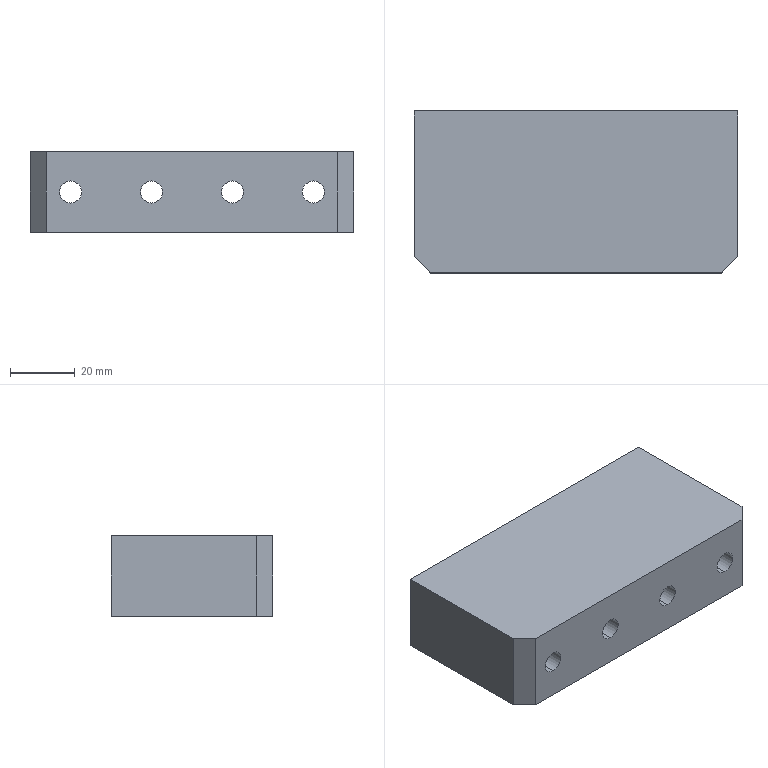Part | SolidWorks | features Chamfer 1, Extrusion 1, HoleWzd 1 | 1 solid | 16 faces | box 100 x 50 x 25 mm | volume 117112 mm3 | cylinder 8 | plane 8 | commonest cylinder face diameters 6.8 x8
STEP:
#1=CARTESIAN_POINT('',(-37.5,-25.,9.1));
#2=VERTEX_POINT('',#1);
#3=CARTESIAN_POINT('',(-37.5,-25.,15.9));
#4=VERTEX_POINT('',#3);
#5=CARTESIAN_POINT('',(-37.5,-25.,12.5));
#6=DIRECTION('',(0.,1.,0.));
#7=DIRECTION('',(0.,0.,1.));
#8=AXIS2_PLACEMENT_3D('',#5,#6,#7);
#9=CIRCLE('',#8,3.4);
#10=EDGE_CURVE('',#2,#4,#9,.T.);
#11=ORIENTED_EDGE('',*,*,#10,.F.);
#12=CARTESIAN_POINT('',(-37.5,25.,9.1));
#13=VERTEX_POINT('',#12);
#14=CARTESIAN_POINT('',(-37.5,25.,9.1));
#15=DIRECTION('',(0.,1.,0.));
#16=VECTOR('',#15,1000.);
#17=LINE('',#14,#16);
#18=EDGE_CURVE('',#2,#13,#17,.T.);
#19=ORIENTED_EDGE('',*,*,#18,.T.);
#20=CARTESIAN_POINT('',(-37.5,25.,15.9));
#21=VERTEX_POINT('',#20);
#22=CARTESIAN_POINT('',(-37.5,25.,12.5));
#23=DIRECTION('',(0.,1.,0.));
#24=DIRECTION('',(0.,0.,1.));
#25=AXIS2_PLACEMENT_3D('',#22,#23,#24);
#26=CIRCLE('',#25,3.4);
#27=EDGE_CURVE('',#13,#21,#26,.T.);
#28=ORIENTED_EDGE('',*,*,#27,.T.);
#29=CARTESIAN_POINT('',(-37.5,25.,15.9));
#30=DIRECTION('',(0.,1.,0.));
#31=VECTOR('',#30,1000.);
#32=LINE('',#29,#31);
#33=EDGE_CURVE('',#4,#21,#32,.T.);
#34=ORIENTED_EDGE('',*,*,#33,.F.);
#35=EDGE_LOOP('',(#11,#19,#28,#34));
#36=FACE_OUTER_BOUND('',#35,.T.);
#37=CARTESIAN_POINT('',(-37.5,25.,12.5));
#38=DIRECTION('',(0.,1.,0.));
#39=DIRECTION('',(0.,0.,1.));
#40=AXIS2_PLACEMENT_3D('',#37,#38,#39);
#41=CYLINDRICAL_SURFACE('',#40,3.4);
#42=ADVANCED_FACE('',(#36),#41,.F.);
#43=CARTESIAN_POINT('',(-12.5,-25.,9.1));
#44=VERTEX_POINT('',#43);
#45=CARTESIAN_POINT('',(-12.5,-25.,15.9));
#46=VERTEX_POINT('',#45);
#47=CARTESIAN_POINT('',(-12.5,-25.,12.5));
#48=DIRECTION('',(0.,1.,0.));
#49=DIRECTION('',(0.,0.,1.));
#50=AXIS2_PLACEMENT_3D('',#47,#48,#49);
#51=CIRCLE('',#50,3.4);
#52=EDGE_CURVE('',#44,#46,#51,.T.);
#53=ORIENTED_EDGE('',*,*,#52,.F.);
#54=CARTESIAN_POINT('',(-12.5,25.,9.1));
#55=VERTEX_POINT('',#54);
#56=CARTESIAN_POINT('',(-12.5,25.,9.1));
#57=DIRECTION('',(0.,1.,0.));
#58=VECTOR('',#57,1000.);
#59=LINE('',#56,#58);
#60=EDGE_CURVE('',#44,#55,#59,.T.);
#61=ORIENTED_EDGE('',*,*,#60,.T.);
#62=CARTESIAN_POINT('',(-12.5,25.,15.9));
#63=VERTEX_POINT('',#62);
#64=CARTESIAN_POINT('',(-12.5,25.,12.5));
#65=DIRECTION('',(0.,1.,0.));
#66=DIRECTION('',(0.,0.,1.));
#67=AXIS2_PLACEMENT_3D('',#64,#65,#66);
#68=CIRCLE('',#67,3.4);
#69=EDGE_CURVE('',#55,#63,#68,.T.);
#70=ORIENTED_EDGE('',*,*,#69,.T.);
#71=CARTESIAN_POINT('',(-12.5,25.,15.9));
#72=DIRECTION('',(0.,1.,0.));
#73=VECTOR('',#72,1000.);
#74=LINE('',#71,#73);
#75=EDGE_CURVE('',#46,#63,#74,.T.);
#76=ORIENTED_EDGE('',*,*,#75,.F.);
#77=EDGE_LOOP('',(#53,#61,#70,#76));
#78=FACE_OUTER_BOUND('',#77,.T.);
#79=CARTESIAN_POINT('',(-12.5,25.,12.5));
#80=DIRECTION('',(0.,1.,0.));
#81=DIRECTION('',(0.,0.,1.));
#82=AXIS2_PLACEMENT_3D('',#79,#80,#81);
#83=CYLINDRICAL_SURFACE('',#82,3.4);
#84=ADVANCED_FACE('',(#78),#83,.F.);
#85=CARTESIAN_POINT('',(12.5,-25.,9.1));
#86=VERTEX_POINT('',#85);
#87=CARTESIAN_POINT('',(12.5,-25.,15.9));
#88=VERTEX_POINT('',#87);
#89=CARTESIAN_POINT('',(12.5,-25.,12.5));
#90=DIRECTION('',(0.,1.,0.));
#91=DIRECTION('',(0.,0.,1.));
#92=AXIS2_PLACEMENT_3D('',#89,#90,#91);
#93=CIRCLE('',#92,3.4);
#94=EDGE_CURVE('',#86,#88,#93,.T.);
#95=ORIENTED_EDGE('',*,*,#94,.F.);
#96=CARTESIAN_POINT('',(12.5,25.,9.1));
#97=VERTEX_POINT('',#96);
#98=CARTESIAN_POINT('',(12.5,25.,9.1));
#99=DIRECTION('',(0.,1.,0.));
#100=VECTOR('',#99,1000.);
#101=LINE('',#98,#100);
#102=EDGE_CURVE('',#86,#97,#101,.T.);
#103=ORIENTED_EDGE('',*,*,#102,.T.);
#104=CARTESIAN_POINT('',(12.5,25.,15.9));
#105=VERTEX_POINT('',#104);
#106=CARTESIAN_POINT('',(12.5,25.,12.5));
#107=DIRECTION('',(0.,1.,0.));
#108=DIRECTION('',(0.,0.,1.));
#109=AXIS2_PLACEMENT_3D('',#106,#107,#108);
#110=CIRCLE('',#109,3.4);
#111=EDGE_CURVE('',#97,#105,#110,.T.);
#112=ORIENTED_EDGE('',*,*,#111,.T.);
#113=CARTESIAN_POINT('',(12.5,25.,15.9));
#114=DIRECTION('',(0.,1.,0.));
#115=VECTOR('',#114,1000.);
#116=LINE('',#113,#115);
#117=EDGE_CURVE('',#88,#105,#116,.T.);
#118=ORIENTED_EDGE('',*,*,#117,.F.);
#119=EDGE_LOOP('',(#95,#103,#112,#118));
#120=FACE_OUTER_BOUND('',#119,.T.);
#121=CARTESIAN_POINT('',(12.5,25.,12.5));
#122=DIRECTION('',(0.,1.,0.));
#123=DIRECTION('',(0.,0.,1.));
#124=AXIS2_PLACEMENT_3D('',#121,#122,#123);
#125=CYLINDRICAL_SURFACE('',#124,3.4);
#126=ADVANCED_FACE('',(#120),#125,.F.);
#127=CARTESIAN_POINT('',(37.5,-25.,9.1));
#128=VERTEX_POINT('',#127);
#129=CARTESIAN_POINT('',(37.5,-25.,15.9));
#130=VERTEX_POINT('',#129);
#131=CARTESIAN_POINT('',(37.5,-25.,12.5));
#132=DIRECTION('',(0.,1.,0.));
#133=DIRECTION('',(0.,0.,1.));
#134=AXIS2_PLACEMENT_3D('',#131,#132,#133);
#135=CIRCLE('',#134,3.4);
#136=EDGE_CURVE('',#128,#130,#135,.T.);
#137=ORIENTED_EDGE('',*,*,#136,.F.);
#138=CARTESIAN_POINT('',(37.5,25.,9.1));
#139=VERTEX_POINT('',#138);
#140=CARTESIAN_POINT('',(37.5,25.,9.1));
#141=DIRECTION('',(0.,1.,0.));
#142=VECTOR('',#141,1000.);
#143=LINE('',#140,#142);
#144=EDGE_CURVE('',#128,#139,#143,.T.);
#145=ORIENTED_EDGE('',*,*,#144,.T.);
#146=CARTESIAN_POINT('',(37.5,25.,15.9));
#147=VERTEX_POINT('',#146);
#148=CARTESIAN_POINT('',(37.5,25.,12.5));
#149=DIRECTION('',(0.,1.,0.));
#150=DIRECTION('',(0.,0.,1.));
#151=AXIS2_PLACEMENT_3D('',#148,#149,#150);
#152=CIRCLE('',#151,3.4);
#153=EDGE_CURVE('',#139,#147,#152,.T.);
#154=ORIENTED_EDGE('',*,*,#153,.T.);
#155=CARTESIAN_POINT('',(37.5,25.,15.9));
#156=DIRECTION('',(0.,1.,0.));
#157=VECTOR('',#156,1000.);
#158=LINE('',#155,#157);
#159=EDGE_CURVE('',#130,#147,#158,.T.);
#160=ORIENTED_EDGE('',*,*,#159,.F.);
#161=EDGE_LOOP('',(#137,#145,#154,#160));
#162=FACE_OUTER_BOUND('',#161,.T.);
#163=CARTESIAN_POINT('',(37.5,25.,12.5));
#164=DIRECTION('',(0.,1.,0.));
#165=DIRECTION('',(0.,0.,1.));
#166=AXIS2_PLACEMENT_3D('',#163,#164,#165);
#167=CYLINDRICAL_SURFACE('',#166,3.4);
#168=ADVANCED_FACE('',(#162),#167,.F.);
#169=CARTESIAN_POINT('',(-37.5,-25.,12.5));
#170=DIRECTION('',(0.,1.,0.));
#171=DIRECTION('',(0.,0.,1.));
#172=AXIS2_PLACEMENT_3D('',#169,#170,#171);
#173=CIRCLE('',#172,3.4);
#174=EDGE_CURVE('',#4,#2,#173,.T.);
#175=ORIENTED_EDGE('',*,*,#174,.T.);
#176=ORIENTED_EDGE('',*,*,#10,.T.);
#177=EDGE_LOOP('',(#175,#176));
#178=FACE_BOUND('',#177,.T.);
#179=CARTESIAN_POINT('',(-12.5,-25.,12.5));
#180=DIRECTION('',(0.,1.,0.));
#181=DIRECTION('',(0.,0.,1.));
#182=AXIS2_PLACEMENT_3D('',#179,#180,#181);
#183=CIRCLE('',#182,3.4);
#184=EDGE_CURVE('',#46,#44,#183,.T.);
#185=ORIENTED_EDGE('',*,*,#184,.T.);
#186=ORIENTED_EDGE('',*,*,#52,.T.);
#187=EDGE_LOOP('',(#185,#186));
#188=FACE_BOUND('',#187,.T.);
#189=CARTESIAN_POINT('',(12.5,-25.,12.5));
#190=DIRECTION('',(0.,1.,0.));
#191=DIRECTION('',(0.,0.,1.));
#192=AXIS2_PLACEMENT_3D('',#189,#190,#191);
#193=CIRCLE('',#192,3.4);
#194=EDGE_CURVE('',#88,#86,#193,.T.);
#195=ORIENTED_EDGE('',*,*,#194,.T.);
#196=ORIENTED_EDGE('',*,*,#94,.T.);
#197=EDGE_LOOP('',(#195,#196));
#198=FACE_BOUND('',#197,.T.);
#199=CARTESIAN_POINT('',(37.5,-25.,12.5));
#200=DIRECTION('',(0.,1.,0.));
#201=DIRECTION('',(0.,0.,1.));
#202=AXIS2_PLACEMENT_3D('',#199,#200,#201);
#203=CIRCLE('',#202,3.4);
#204=EDGE_CURVE('',#130,#128,#203,.T.);
#205=ORIENTED_EDGE('',*,*,#204,.T.);
#206=ORIENTED_EDGE('',*,*,#136,.T.);
#207=EDGE_LOOP('',(#205,#206));
#208=FACE_BOUND('',#207,.T.);
#209=CARTESIAN_POINT('',(-45.,-25.,25.));
#210=VERTEX_POINT('',#209);
#211=CARTESIAN_POINT('',(45.,-25.,25.));
#212=VERTEX_POINT('',#211);
#213=CARTESIAN_POINT('',(-50.,-25.,25.));
#214=DIRECTION('',(1.,0.,0.));
#215=VECTOR('',#214,1000.);
#216=LINE('',#213,#215);
#217=EDGE_CURVE('',#210,#212,#216,.T.);
#218=ORIENTED_EDGE('',*,*,#217,.F.);
#219=CARTESIAN_POINT('',(-45.,-25.,0.));
#220=VERTEX_POINT('',#219);
#221=CARTESIAN_POINT('',(-45.,-25.,25.));
#222=DIRECTION('',(0.,0.,-1.));
#223=VECTOR('',#222,1000.);
#224=LINE('',#221,#223);
#225=EDGE_CURVE('',#210,#220,#224,.T.);
#226=ORIENTED_EDGE('',*,*,#225,.T.);
#227=CARTESIAN_POINT('',(45.,-25.,0.));
#228=VERTEX_POINT('',#227);
#229=CARTESIAN_POINT('',(-50.,-25.,0.));
#230=DIRECTION('',(1.,0.,0.));
#231=VECTOR('',#230,1000.);
#232=LINE('',#229,#231);
#233=EDGE_CURVE('',#220,#228,#232,.T.);
#234=ORIENTED_EDGE('',*,*,#233,.T.);
#235=CARTESIAN_POINT('',(45.,-25.,25.));
#236=DIRECTION('',(0.,0.,1.));
#237=VECTOR('',#236,1000.);
#238=LINE('',#235,#237);
#239=EDGE_CURVE('',#228,#212,#238,.T.);
#240=ORIENTED_EDGE('',*,*,#239,.T.);
#241=EDGE_LOOP('',(#218,#226,#234,#240));
#242=FACE_OUTER_BOUND('',#241,.T.);
#243=CARTESIAN_POINT('',(-50.,-25.,25.));
#244=DIRECTION('',(0.,1.,0.));
#245=DIRECTION('',(0.,0.,1.));
#246=AXIS2_PLACEMENT_3D('',#243,#244,#245);
#247=PLANE('',#246);
#248=ADVANCED_FACE('',(#178,#188,#198,#208,#242),#247,.F.);
#249=CARTESIAN_POINT('',(50.,25.,25.));
#250=VERTEX_POINT('',#249);
#251=CARTESIAN_POINT('',(50.,-20.,25.));
#252=VERTEX_POINT('',#251);
#253=CARTESIAN_POINT('',(50.,25.,25.));
#254=DIRECTION('',(0.,-1.,0.));
#255=VECTOR('',#254,1000.);
#256=LINE('',#253,#255);
#257=EDGE_CURVE('',#250,#252,#256,.T.);
#258=ORIENTED_EDGE('',*,*,#257,.T.);
#259=CARTESIAN_POINT('',(50.,-20.,0.));
#260=VERTEX_POINT('',#259);
#261=CARTESIAN_POINT('',(50.,-20.,0.));
#262=DIRECTION('',(0.,0.,-1.));
#263=VECTOR('',#262,1000.);
#264=LINE('',#261,#263);
#265=EDGE_CURVE('',#252,#260,#264,.T.);
#266=ORIENTED_EDGE('',*,*,#265,.T.);
#267=CARTESIAN_POINT('',(50.,25.,0.));
#268=VERTEX_POINT('',#267);
#269=CARTESIAN_POINT('',(50.,25.,0.));
#270=DIRECTION('',(0.,-1.,0.));
#271=VECTOR('',#270,1000.);
#272=LINE('',#269,#271);
#273=EDGE_CURVE('',#268,#260,#272,.T.);
#274=ORIENTED_EDGE('',*,*,#273,.F.);
#275=CARTESIAN_POINT('',(50.,25.,25.));
#276=DIRECTION('',(0.,0.,-1.));
#277=VECTOR('',#276,1000.);
#278=LINE('',#275,#277);
#279=EDGE_CURVE('',#250,#268,#278,.T.);
#280=ORIENTED_EDGE('',*,*,#279,.F.);
#281=EDGE_LOOP('',(#258,#266,#274,#280));
#282=FACE_OUTER_BOUND('',#281,.T.);
#283=CARTESIAN_POINT('',(50.,25.,25.));
#284=DIRECTION('',(1.,0.,0.));
#285=DIRECTION('',(0.,1.,0.));
#286=AXIS2_PLACEMENT_3D('',#283,#284,#285);
#287=PLANE('',#286);
#288=ADVANCED_FACE('',(#282),#287,.T.);
#289=CARTESIAN_POINT('',(-37.5,25.,12.5));
#290=DIRECTION('',(0.,1.,0.));
#291=DIRECTION('',(0.,0.,1.));
#292=AXIS2_PLACEMENT_3D('',#289,#290,#291);
#293=CIRCLE('',#292,3.4);
#294=EDGE_CURVE('',#21,#13,#293,.T.);
#295=ORIENTED_EDGE('',*,*,#294,.F.);
#296=ORIENTED_EDGE('',*,*,#27,.F.);
#297=EDGE_LOOP('',(#295,#296));
#298=FACE_BOUND('',#297,.T.);
#299=CARTESIAN_POINT('',(-12.5,25.,12.5));
#300=DIRECTION('',(0.,1.,0.));
#301=DIRECTION('',(0.,0.,1.));
#302=AXIS2_PLACEMENT_3D('',#299,#300,#301);
#303=CIRCLE('',#302,3.4);
#304=EDGE_CURVE('',#63,#55,#303,.T.);
#305=ORIENTED_EDGE('',*,*,#304,.F.);
#306=ORIENTED_EDGE('',*,*,#69,.F.);
#307=EDGE_LOOP('',(#305,#306));
#308=FACE_BOUND('',#307,.T.);
#309=CARTESIAN_POINT('',(12.5,25.,12.5));
#310=DIRECTION('',(0.,1.,0.));
#311=DIRECTION('',(0.,0.,1.));
#312=AXIS2_PLACEMENT_3D('',#309,#310,#311);
#313=CIRCLE('',#312,3.4);
#314=EDGE_CURVE('',#105,#97,#313,.T.);
#315=ORIENTED_EDGE('',*,*,#314,.F.);
#316=ORIENTED_EDGE('',*,*,#111,.F.);
#317=EDGE_LOOP('',(#315,#316));
#318=FACE_BOUND('',#317,.T.);
#319=CARTESIAN_POINT('',(37.5,25.,12.5));
#320=DIRECTION('',(0.,1.,0.));
#321=DIRECTION('',(0.,0.,1.));
#322=AXIS2_PLACEMENT_3D('',#319,#320,#321);
#323=CIRCLE('',#322,3.4);
#324=EDGE_CURVE('',#147,#139,#323,.T.);
#325=ORIENTED_EDGE('',*,*,#324,.F.);
#326=ORIENTED_EDGE('',*,*,#153,.F.);
#327=EDGE_LOOP('',(#325,#326));
#328=FACE_BOUND('',#327,.T.);
#329=CARTESIAN_POINT('',(-50.,25.,0.));
#330=VERTEX_POINT('',#329);
#331=CARTESIAN_POINT('',(-50.,25.,0.));
#332=DIRECTION('',(1.,0.,0.));
#333=VECTOR('',#332,1000.);
#334=LINE('',#331,#333);
#335=EDGE_CURVE('',#330,#268,#334,.T.);
#336=ORIENTED_EDGE('',*,*,#335,.F.);
#337=CARTESIAN_POINT('',(-50.,25.,25.));
#338=VERTEX_POINT('',#337);
#339=CARTESIAN_POINT('',(-50.,25.,25.));
#340=DIRECTION('',(0.,0.,-1.));
#341=VECTOR('',#340,1000.);
#342=LINE('',#339,#341);
#343=EDGE_CURVE('',#338,#330,#342,.T.);
#344=ORIENTED_EDGE('',*,*,#343,.F.);
#345=CARTESIAN_POINT('',(-50.,25.,25.));
#346=DIRECTION('',(1.,0.,0.));
#347=VECTOR('',#346,1000.);
#348=LINE('',#345,#347);
#349=EDGE_CURVE('',#338,#250,#348,.T.);
#350=ORIENTED_EDGE('',*,*,#349,.T.);
#351=ORIENTED_EDGE('',*,*,#279,.T.);
#352=EDGE_LOOP('',(#336,#344,#350,#351));
#353=FACE_OUTER_BOUND('',#352,.T.);
#354=CARTESIAN_POINT('',(-50.,25.,25.));
#355=DIRECTION('',(0.,1.,0.));
#356=DIRECTION('',(0.,0.,1.));
#357=AXIS2_PLACEMENT_3D('',#354,#355,#356);
#358=PLANE('',#357);
#359=ADVANCED_FACE('',(#298,#308,#318,#328,#353),#358,.T.);
#360=CARTESIAN_POINT('',(-50.,-20.,0.));
#361=VERTEX_POINT('',#360);
#362=CARTESIAN_POINT('',(-50.,25.,0.));
#363=DIRECTION('',(0.,-1.,0.));
#364=VECTOR('',#363,1000.);
#365=LINE('',#362,#364);
#366=EDGE_CURVE('',#330,#361,#365,.T.);
#367=ORIENTED_EDGE('',*,*,#366,.T.);
#368=CARTESIAN_POINT('',(-50.,-20.,25.));
#369=VERTEX_POINT('',#368);
#370=CARTESIAN_POINT('',(-50.,-20.,25.));
#371=DIRECTION('',(0.,0.,1.));
#372=VECTOR('',#371,1000.);
#373=LINE('',#370,#372);
#374=EDGE_CURVE('',#361,#369,#373,.T.);
#375=ORIENTED_EDGE('',*,*,#374,.T.);
#376=CARTESIAN_POINT('',(-50.,25.,25.));
#377=DIRECTION('',(0.,-1.,0.));
#378=VECTOR('',#377,1000.);
#379=LINE('',#376,#378);
#380=EDGE_CURVE('',#338,#369,#379,.T.);
#381=ORIENTED_EDGE('',*,*,#380,.F.);
#382=ORIENTED_EDGE('',*,*,#343,.T.);
#383=EDGE_LOOP('',(#367,#375,#381,#382));
#384=FACE_OUTER_BOUND('',#383,.T.);
#385=CARTESIAN_POINT('',(-50.,25.,25.));
#386=DIRECTION('',(1.,0.,0.));
#387=DIRECTION('',(0.,1.,0.));
#388=AXIS2_PLACEMENT_3D('',#385,#386,#387);
#389=PLANE('',#388);
#390=ADVANCED_FACE('',(#384),#389,.F.);
#391=ORIENTED_EDGE('',*,*,#380,.T.);
#392=CARTESIAN_POINT('',(-45.,-25.,25.));
#393=DIRECTION('',(0.7071,-0.7071,0.));
#394=VECTOR('',#393,1000.);
#395=LINE('',#392,#394);
#396=EDGE_CURVE('',#369,#210,#395,.T.);
#397=ORIENTED_EDGE('',*,*,#396,.T.);
#398=ORIENTED_EDGE('',*,*,#217,.T.);
#399=CARTESIAN_POINT('',(50.,-20.,25.));
#400=DIRECTION('',(0.7071,0.7071,0.));
#401=VECTOR('',#400,1000.);
#402=LINE('',#399,#401);
#403=EDGE_CURVE('',#212,#252,#402,.T.);
#404=ORIENTED_EDGE('',*,*,#403,.T.);
#405=ORIENTED_EDGE('',*,*,#257,.F.);
#406=ORIENTED_EDGE('',*,*,#349,.F.);
#407=EDGE_LOOP('',(#391,#397,#398,#404,#405,#406));
#408=FACE_OUTER_BOUND('',#407,.T.);
#409=CARTESIAN_POINT('',(0.,0.,25.));
#410=DIRECTION('',(0.,0.,-1.));
#411=DIRECTION('',(-1.,0.,0.));
#412=AXIS2_PLACEMENT_3D('',#409,#410,#411);
#413=PLANE('',#412);
#414=ADVANCED_FACE('',(#408),#413,.F.);
#415=ORIENTED_EDGE('',*,*,#233,.F.);
#416=CARTESIAN_POINT('',(-35.,-35.,0.));
#417=DIRECTION('',(-0.7071,0.7071,0.));
#418=VECTOR('',#417,1000.);
#419=LINE('',#416,#418);
#420=EDGE_CURVE('',#220,#361,#419,.T.);
#421=ORIENTED_EDGE('',*,*,#420,.T.);
#422=ORIENTED_EDGE('',*,*,#366,.F.);
#423=ORIENTED_EDGE('',*,*,#335,.T.);
#424=ORIENTED_EDGE('',*,*,#273,.T.);
#425=CARTESIAN_POINT('',(35.,-35.,0.));
#426=DIRECTION('',(-0.7071,-0.7071,0.));
#427=VECTOR('',#426,1000.);
#428=LINE('',#425,#427);
#429=EDGE_CURVE('',#260,#228,#428,.T.);
#430=ORIENTED_EDGE('',*,*,#429,.T.);
#431=EDGE_LOOP('',(#415,#421,#422,#423,#424,#430));
#432=FACE_OUTER_BOUND('',#431,.T.);
#433=CARTESIAN_POINT('',(0.,0.,0.));
#434=DIRECTION('',(0.,0.,-1.));
#435=DIRECTION('',(-1.,0.,0.));
#436=AXIS2_PLACEMENT_3D('',#433,#434,#435);
#437=PLANE('',#436);
#438=ADVANCED_FACE('',(#432),#437,.T.);
#439=ORIENTED_EDGE('',*,*,#144,.F.);
#440=ORIENTED_EDGE('',*,*,#204,.F.);
#441=ORIENTED_EDGE('',*,*,#159,.T.);
#442=ORIENTED_EDGE('',*,*,#324,.T.);
#443=EDGE_LOOP('',(#439,#440,#441,#442));
#444=FACE_OUTER_BOUND('',#443,.T.);
#445=CARTESIAN_POINT('',(37.5,25.,12.5));
#446=DIRECTION('',(0.,1.,0.));
#447=DIRECTION('',(0.,0.,1.));
#448=AXIS2_PLACEMENT_3D('',#445,#446,#447);
#449=CYLINDRICAL_SURFACE('',#448,3.4);
#450=ADVANCED_FACE('',(#444),#449,.F.);
#451=ORIENTED_EDGE('',*,*,#102,.F.);
#452=ORIENTED_EDGE('',*,*,#194,.F.);
#453=ORIENTED_EDGE('',*,*,#117,.T.);
#454=ORIENTED_EDGE('',*,*,#314,.T.);
#455=EDGE_LOOP('',(#451,#452,#453,#454));
#456=FACE_OUTER_BOUND('',#455,.T.);
#457=CARTESIAN_POINT('',(12.5,25.,12.5));
#458=DIRECTION('',(0.,1.,0.));
#459=DIRECTION('',(0.,0.,1.));
#460=AXIS2_PLACEMENT_3D('',#457,#458,#459);
#461=CYLINDRICAL_SURFACE('',#460,3.4);
#462=ADVANCED_FACE('',(#456),#461,.F.);
#463=ORIENTED_EDGE('',*,*,#60,.F.);
#464=ORIENTED_EDGE('',*,*,#184,.F.);
#465=ORIENTED_EDGE('',*,*,#75,.T.);
#466=ORIENTED_EDGE('',*,*,#304,.T.);
#467=EDGE_LOOP('',(#463,#464,#465,#466));
#468=FACE_OUTER_BOUND('',#467,.T.);
#469=CARTESIAN_POINT('',(-12.5,25.,12.5));
#470=DIRECTION('',(0.,1.,0.));
#471=DIRECTION('',(0.,0.,1.));
#472=AXIS2_PLACEMENT_3D('',#469,#470,#471);
#473=CYLINDRICAL_SURFACE('',#472,3.4);
#474=ADVANCED_FACE('',(#468),#473,.F.);
#475=ORIENTED_EDGE('',*,*,#18,.F.);
#476=ORIENTED_EDGE('',*,*,#174,.F.);
#477=ORIENTED_EDGE('',*,*,#33,.T.);
#478=ORIENTED_EDGE('',*,*,#294,.T.);
#479=EDGE_LOOP('',(#475,#476,#477,#478));
#480=FACE_OUTER_BOUND('',#479,.T.);
#481=CARTESIAN_POINT('',(-37.5,25.,12.5));
#482=DIRECTION('',(0.,1.,0.));
#483=DIRECTION('',(0.,0.,1.));
#484=AXIS2_PLACEMENT_3D('',#481,#482,#483);
#485=CYLINDRICAL_SURFACE('',#484,3.4);
#486=ADVANCED_FACE('',(#480),#485,.F.);
#487=ORIENTED_EDGE('',*,*,#396,.F.);
#488=ORIENTED_EDGE('',*,*,#374,.F.);
#489=ORIENTED_EDGE('',*,*,#420,.F.);
#490=ORIENTED_EDGE('',*,*,#225,.F.);
#491=EDGE_LOOP('',(#487,#488,#489,#490));
#492=FACE_OUTER_BOUND('',#491,.T.);
#493=CARTESIAN_POINT('',(-45.,-25.,25.));
#494=DIRECTION('',(0.7071,0.7071,0.));
#495=DIRECTION('',(0.,0.,-1.));
#496=AXIS2_PLACEMENT_3D('',#493,#494,#495);
#497=PLANE('',#496);
#498=ADVANCED_FACE('',(#492),#497,.F.);
#499=ORIENTED_EDGE('',*,*,#403,.F.);
#500=ORIENTED_EDGE('',*,*,#239,.F.);
#501=ORIENTED_EDGE('',*,*,#429,.F.);
#502=ORIENTED_EDGE('',*,*,#265,.F.);
#503=EDGE_LOOP('',(#499,#500,#501,#502));
#504=FACE_OUTER_BOUND('',#503,.T.);
#505=CARTESIAN_POINT('',(50.,-20.,25.));
#506=DIRECTION('',(0.7071,-0.7071,0.));
#507=DIRECTION('',(0.,0.,1.));
#508=AXIS2_PLACEMENT_3D('',#505,#506,#507);
#509=PLANE('',#508);
#510=ADVANCED_FACE('',(#504),#509,.T.);
#511=CLOSED_SHELL('',(#42,#84,#126,#168,#248,#288,#359,#390,#414,#438,#450,#462,#474,#486,#498,#510));
#512=MANIFOLD_SOLID_BREP('',#511);
#513=CARTESIAN_POINT('',(0.,0.,0.));
#514=DIRECTION('',(0.,0.,1.));
#515=DIRECTION('',(1.,0.,0.));
#516=AXIS2_PLACEMENT_3D('',#513,#514,#515);
#517=(LENGTH_UNIT()NAMED_UNIT(*)SI_UNIT(.MILLI.,.METRE.));
#518=UNCERTAINTY_MEASURE_WITH_UNIT(LENGTH_MEASURE(0.00001),#517,'','');
#519=(NAMED_UNIT(*)PLANE_ANGLE_UNIT()SI_UNIT($,.RADIAN.));
#520=(NAMED_UNIT(*)SI_UNIT($,.STERADIAN.)SOLID_ANGLE_UNIT());
#521=(GEOMETRIC_REPRESENTATION_CONTEXT(3)GLOBAL_UNCERTAINTY_ASSIGNED_CONTEXT((#518))GLOBAL_UNIT_ASSIGNED_CONTEXT((#517,#519,#520))REPRESENTATION_CONTEXT('',''));
#522=ADVANCED_BREP_SHAPE_REPRESENTATION('',(#512,#516),#521);